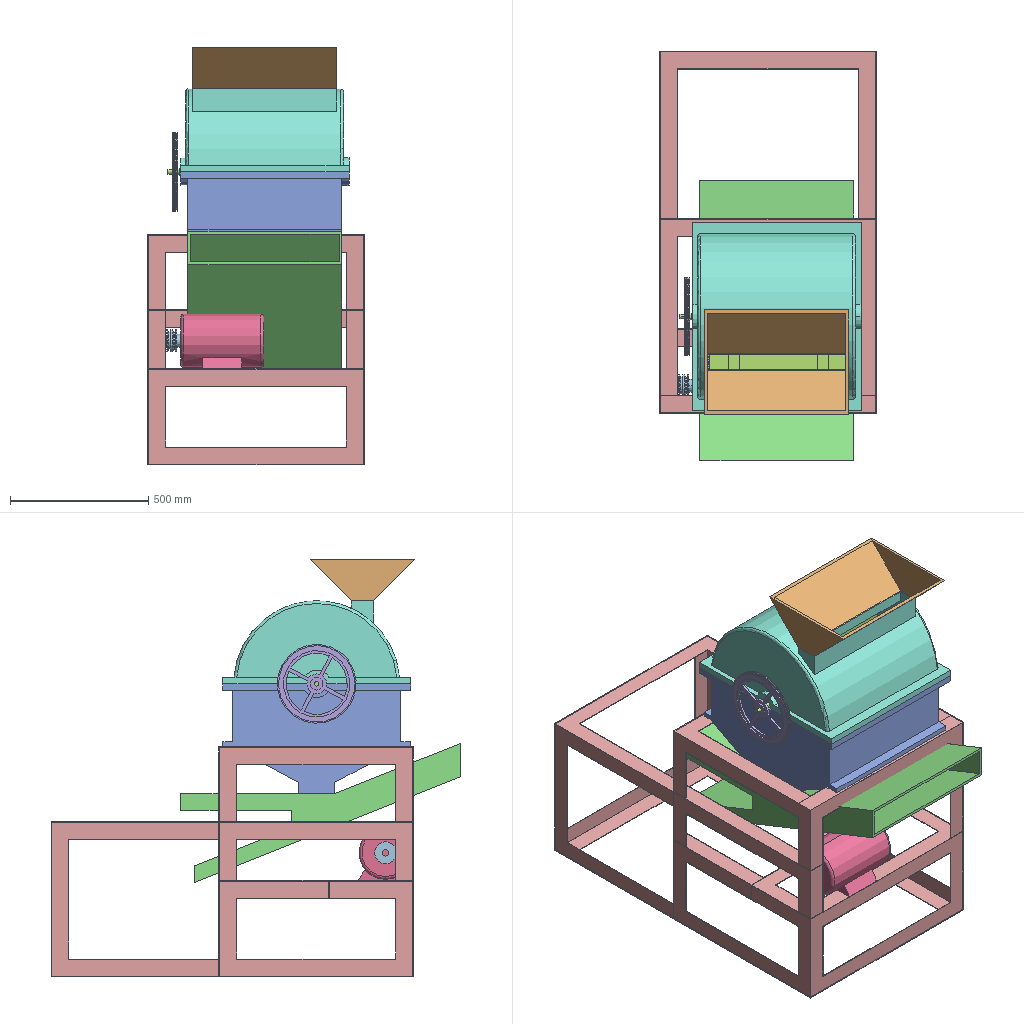Assembly | SolidWorks | 10 different items | 10 placed | box 780 x 1480 x 1508 mm
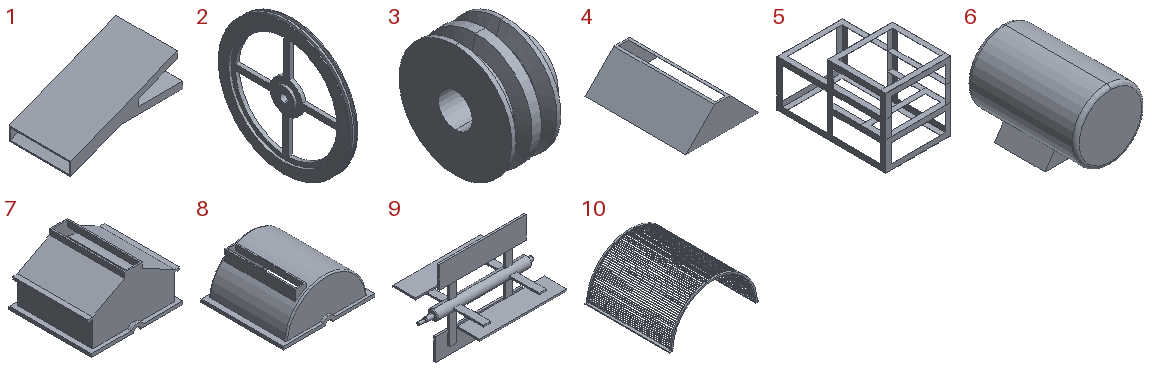Parts list (item | quantity | size | volume | features):
1 | x1 | 1012 x 556 x 502.062 mm | 17769290 mm3 | features Extrusion 1, ICE 1, Shell 1
2 | x1 | 18 x 285 x 285 mm | 431975 mm3 | features ICE 6, CirPattern 1, Revolution 1
3 | x1 | 48.997 x 80 x 80 mm | 144144 mm3 | features Revolution 1
4 | x1 | 376 x 520 x 150 mm | 2791226 mm3 | features Extrusion 1, MirrorPattern 1, Shell 1
5 | x1 | 780 x 1308 x 830 mm | 4147538 mm3 | features ICE 9, MirrorPattern 3, Extrusion 1
6 | x1 | 200 x 350 x 196 mm | 9129651 mm3 | features ICE 2, Extrusion 1, Fillet 1
7 | x1 | 677.491 x 608 x 396.469 mm | 20641288 mm3 | features ICE 5, MirrorPattern 4, Extrusion 1
8 | x1 | 677.491 x 608 x 300 mm | 10187902 mm3 | features ICE 11, MirrorPattern 4, Extrusion 1, Fillet 1
9 | x1 | 650 x 499.161 x 499.161 mm | 4694560 mm3 | features ICE 2, Chamfer 1, CirPattern 1, RefAxis 1, Revolution 1
10 | x1 | 570 x 540 x 276.117 mm | 657758 mm3 | features ICE 2, MirrorPattern 2, CirPattern 1, Extrusion 1, RefAxis 1
Mates (type | each side: item.copy, entity, surface, feature):
Coincident | 5.1 face plane Boss-Extrude2 | 7.1 face plane Mirror8
DistanceDim | 7.1 face plane Boss-Extrude1 | 5.1 face plane Mirror4
DistanceDim | 7.1 face plane Mirror8 | 5.1 face plane Boss-Extrude1
Concentric | 7.1 face cylinder Cut-Extrude1 | 9.1 face cylinder Revolve1
DistanceDim | 9.1 face plane Revolve1 | 7.1 face plane Boss-Extrude2
Concentric | 7.1 face cylinder Mirror8 | 10.1 face cylinder Mirror3
Coincident | 7.1 face plane Boss-Extrude1 | 10.1 face plane Boss-Extrude1
Coincident | 7.1 face plane Mirror2 | 10.1 face plane Boss-Extrude1
Concentric | 9.1 face cylinder Revolve1 | 8.1 face cylinder Cut-Extrude1
Coincident | 7.1 face plane Mirror3 | 8.1 face plane Mirror3
Coincident | 8.1 face plane Boss-Extrude9 | 4.1 face plane Boss-Extrude1 | 2 times
Coincident | 8.1 edge | 4.1 edge
Concentric | 9.1 face cylinder Revolve1 | 2.1 face cylinder Cut-Extrude3
DistanceDim | 2.1 face plane Boss-Extrude2 | 9.1 face plane Revolve1
Coincident | 7.1 face plane Boss-Extrude1 | 1.1 face plane Boss-Extrude1 | 2 times
Coincident | 7.1 edge | 1.1 edge
Parallel | 9.1 face cylinder Revolve1 | 6.1 face cylinder Boss-Extrude1
Coincident | 8.1 face plane Boss-Extrude3 | 6.1 face plane Boss-Extrude1
Coincident | 5.1 face plane Boss-Extrude1 | 6.1 edge
Coincident | 5.1 face plane Boss-Extrude9 | 6.1 face plane Boss-Extrude3
Concentric | 6.1 face cylinder Boss-Extrude2 | 3.1 face cylinder Revolve1
Coincident | 6.1 face plane Boss-Extrude2 | 3.1 face plane Revolve1